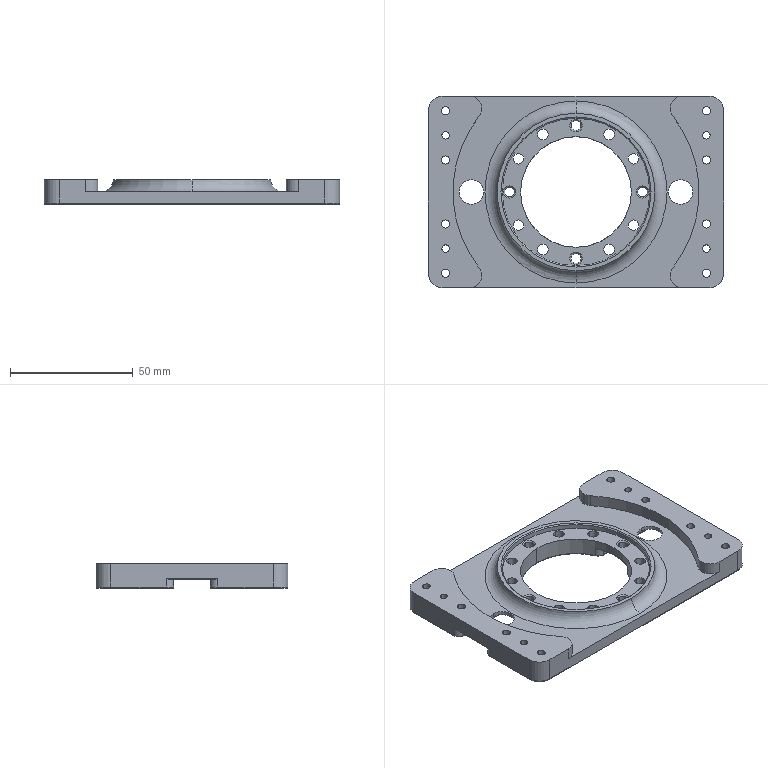NC program | NX | posted with a generic post | part box 120 x 78 x 10 mm
Whole program:
N10 G17 G21 G94 G90
(HOLE_MILLING_1_COPY_1 , TOOL : D3)
N12 T17 M6
N14 G54
N16 G17 G0 G90 X-47.5 Y0. B0. C0. S9500 M3
N18 G43 Z30. H17
N20 Z0.5
N22 G94 G3 X-47.95 Y0.45 R0.45 F1250.
N24 X-48.4 Y0. R0.45
N26 X-48.4 Y0. Z0.25 I0.9 J0.
N28 X-48.4 Y0. Z0. I0.9 J0.
N30 X-48.4 Y0. Z-0.25 I0.9 J0.
N32 X-48.4 Y0. Z-0.5 I0.9 J0.
N34 X-48.4 Y0. Z-0.75 I0.9 J0.
N36 X-48.4 Y0. Z-1. I0.9 J0.
N38 X-48.4 Y0. Z-1.25 I0.9 J0.
N40 X-48.4 Y0. Z-1.5 I0.9 J0.
N42 X-48.4 Y0. Z-1.75 I0.9 J0.
N44 X-48.4 Y0. Z-2. I0.9 J0.
N46 X-48.4 Y0. Z-2.25 I0.9 J0.
N48 X-48.4 Y0. Z-2.5 I0.9 J0.
N50 X-48.4 Y0. Z-2.75 I0.9 J0.
N52 X-48.4 Y0. Z-3. I0.9 J0.
N54 X-48.4 Y0. Z-3.25 I0.9 J0.
N56 X-48.4 Y0. Z-3.5 I0.9 J0.
N58 X-48.4 Y0. Z-3.75 I0.9 J0.
N60 X-48.4 Y0. Z-4. I0.9 J0.
N62 X-48.4 Y0. Z-4.25 I0.9 J0.
N64 X-48.4 Y0. Z-4.5 I0.9 J0.
N66 X-48.4 Y0. Z-4.75 I0.9 J0.
N68 X-48.4 Y0. Z-5. I0.9 J0.
N70 X-48.4 Y0. Z-5.25 I0.9 J0.
N72 X-48.4 Y0. Z-5.5 I0.9 J0.
N74 X-48.4 Y0. Z-5.75 I0.9 J0.
N76 X-48.4 Y0. Z-6. I0.9 J0.
N78 X-48.4 Y0. Z-6.25 I0.9 J0.
N80 X-48.4 Y0. Z-6.5 I0.9 J0.
N82 X-48.4 Y0. Z-6.75 I0.9 J0.
N84 X-48.4 Y0. Z-7. I0.9 J0.
N86 X-48.4 Y0. Z-7.25 I0.9 J0.
N88 X-48.4 Y0. Z-7.5 I0.9 J0.
N90 X-48.4 Y0. Z-7.75 I0.9 J0.
N92 X-48.4 Y0. Z-8. I0.9 J0.
N94 X-48.4 Y0. Z-8.25 I0.9 J0.
N96 X-48.4 Y0. Z-8.5 I0.9 J0.
N98 X-48.4 Y0. Z-8.75 I0.9 J0.
N100 X-48.4 Y0. Z-9. I0.9 J0.
N102 X-48.4 Y0. Z-9.25 I0.9 J0.
N104 X-48.4 Y0. Z-9.5 I0.9 J0.
N106 X-48.4 Y0. Z-9.75 I0.9 J0.
N108 X-48.4 Y0. Z-10. I0.9 J0.
N110 X-47.5 Y-0.9 R0.9
N112 X-48.4 Y0. R-0.9
N114 X-47.95 Y-0.45 R0.45
N116 X-47.5 Y0. R0.45
N118 G0 Z30.
N120 X47.5
N122 Z0.5
N124 G3 X47.05 Y0.45 R0.45
N126 X46.6 Y0. R0.45
N128 X46.6 Y0. Z0.25 I0.9 J0.
N130 X46.6 Y0. Z0. I0.9 J0.
N132 X46.6 Y0. Z-0.25 I0.9 J0.
N134 X46.6 Y0. Z-0.5 I0.9 J0.
N136 X46.6 Y0. Z-0.75 I0.9 J0.
N138 X46.6 Y0. Z-1. I0.9 J0.
N140 X46.6 Y0. Z-1.25 I0.9 J0.
N142 X46.6 Y0. Z-1.5 I0.9 J0.
N144 X46.6 Y0. Z-1.75 I0.9 J0.
N146 X46.6 Y0. Z-2. I0.9 J0.
N148 X46.6 Y0. Z-2.25 I0.9 J0.
N150 X46.6 Y0. Z-2.5 I0.9 J0.
N152 X46.6 Y0. Z-2.75 I0.9 J0.
N154 X46.6 Y0. Z-3. I0.9 J0.
N156 X46.6 Y0. Z-3.25 I0.9 J0.
N158 X46.6 Y0. Z-3.5 I0.9 J0.
N160 X46.6 Y0. Z-3.75 I0.9 J0.
N162 X46.6 Y0. Z-4. I0.9 J0.
N164 X46.6 Y0. Z-4.25 I0.9 J0.
N166 X46.6 Y0. Z-4.5 I0.9 J0.
N168 X46.6 Y0. Z-4.75 I0.9 J0.
N170 X46.6 Y0. Z-5. I0.9 J0.
N172 X46.6 Y0. Z-5.25 I0.9 J0.
N174 X46.6 Y0. Z-5.5 I0.9 J0.
N176 X46.6 Y0. Z-5.75 I0.9 J0.
N178 X46.6 Y0. Z-6. I0.9 J0.
N180 X46.6 Y0. Z-6.25 I0.9 J0.
N182 X46.6 Y0. Z-6.5 I0.9 J0.
N184 X46.6 Y0. Z-6.75 I0.9 J0.
N186 X46.6 Y0. Z-7. I0.9 J0.
N188 X46.6 Y0. Z-7.25 I0.9 J0.
N190 X46.6 Y0. Z-7.5 I0.9 J0.
N192 X46.6 Y0. Z-7.75 I0.9 J0.
N194 X46.6 Y0. Z-8. I0.9 J0.
N196 X46.6 Y0. Z-8.25 I0.9 J0.
N198 X46.6 Y0. Z-8.5 I0.9 J0.
N200 X46.6 Y0. Z-8.75 I0.9 J0.
N202 X46.6 Y0. Z-9. I0.9 J0.
N204 X46.6 Y0. Z-9.25 I0.9 J0.
N206 X46.6 Y0. Z-9.5 I0.9 J0.
N208 X46.6 Y0. Z-9.75 I0.9 J0.
N210 X46.6 Y0. Z-10. I0.9 J0.
N212 X47.5 Y-0.9 R0.9
N214 X46.6 Y0. R-0.9
N216 X47.05 Y-0.45 R0.45
N218 X47.5 Y0. R0.45
N220 G0 Z30.
N222 M5
(ZLEVEL_PROFILE_COPY_1_COPY_COPY_1_COPY , TOOL : D6A45)
N224 T01 M6
N226 G54
N228 G17 G0 G90 X-46.138 Y1.38 B0. C0. S9500 M3
N230 G43 Z30. H1
N232 Z2.646
N234 G94 G1 Z-0.354 F1000.
N236 X-46.98 Y2.839
N238 G3 X-47.5 Y3.139 R0.6
N240 X-50.639 Y0. R3.139 F1200.
N242 X-47.5 Y3.139 R-3.139
N244 G1 X-47.731 Y3.123 Z-0.357
N246 X-47.961 Y3.098 Z-0.361
N248 X-48.187 Y3.048 Z-0.364
N250 X-48.41 Y2.989 Z-0.368
N252 X-48.626 Y2.907 Z-0.371
N254 X-48.837 Y2.817 Z-0.375
N256 X-49.038 Y2.704 Z-0.378
N258 X-49.234 Y2.583 Z-0.382
N260 X-49.415 Y2.443 Z-0.385
N262 X-49.59 Y2.294 Z-0.389
N264 X-49.749 Y2.129 Z-0.392
N266 X-49.9 Y1.957 Z-0.396
N268 X-50.032 Y1.771 Z-0.399
N270 X-50.156 Y1.579 Z-0.403
N272 X-50.259 Y1.375 Z-0.406
N274 X-50.353 Y1.168 Z-0.41
N276 X-50.424 Y0.952 Z-0.413
N278 X-50.487 Y0.733 Z-0.417
N280 X-50.536 Y0.47 Z-0.421
N282 X-50.556 Y0.285 Z-0.423
N284 X-50.561 Y0.059 Z-0.427
N286 X-50.558 Y-0.168 Z-0.43
N288 X-50.53 Y-0.392 Z-0.434
N290 X-50.493 Y-0.615 Z-0.437
N292 X-50.432 Y-0.832 Z-0.441
N294 X-50.363 Y-1.046 Z-0.444
N296 X-50.271 Y-1.254 Z-0.448
N298 X-50.169 Y-1.458 Z-0.451
N300 X-50.047 Y-1.65 Z-0.455
N302 X-49.917 Y-1.836 Z-0.458
N304 X-49.767 Y-2.006 Z-0.461
N306 X-49.611 Y-2.17 Z-0.465
N308 X-49.439 Y-2.316 Z-0.468
N310 X-49.26 Y-2.455 Z-0.472
N312 X-49.068 Y-2.573 Z-0.475
N314 X-48.872 Y-2.684 Z-0.479
N316 X-48.664 Y-2.772 Z-0.482
N318 X-48.454 Y-2.852 Z-0.486
N320 X-48.237 Y-2.908 Z-0.489
N322 X-48.017 Y-2.955 Z-0.492
N324 X-47.794 Y-2.979 Z-0.496
N326 X-47.571 Y-2.993 Z-0.499
N328 X-47.348 Y-2.983 Z-0.503
N330 X-47.125 Y-2.963 Z-0.506
N332 X-46.906 Y-2.919 Z-0.509
N334 X-46.689 Y-2.868 Z-0.513
N336 X-46.424 Y-2.774 Z-0.517
N338 X-46.274 Y-2.708 Z-0.52
N340 X-46.079 Y-2.603 Z-0.523
N342 X-45.887 Y-2.49 Z-0.526
N344 X-45.711 Y-2.356 Z-0.53
N346 X-45.539 Y-2.217 Z-0.533
N348 X-45.384 Y-2.059 Z-0.537
N350 X-45.235 Y-1.895 Z-0.54
N352 X-45.106 Y-1.717 Z-0.543
N354 X-44.984 Y-1.533 Z-0.547
N356 X-44.883 Y-1.338 Z-0.55
N358 X-44.79 Y-1.138 Z-0.553
N360 X-44.719 Y-0.93 Z-0.557
N362 X-44.657 Y-0.72 Z-0.56
N364 X-44.619 Y-0.504 Z-0.563
N366 X-44.588 Y-0.288 Z-0.567
N368 X-44.582 Y-0.069 Z-0.57
N370 X-44.584 Y0.149 Z-0.573
N372 X-44.611 Y0.366 Z-0.577
N374 X-44.646 Y0.581 Z-0.58
N376 X-44.704 Y0.79 Z-0.583
N378 X-44.77 Y0.998 Z-0.587
N380 X-44.859 Y1.196 Z-0.59
N382 X-44.955 Y1.39 Z-0.593
N384 X-45.072 Y1.572 Z-0.597
N386 X-45.196 Y1.75 Z-0.6
N388 X-45.339 Y1.912 Z-0.603
N390 X-45.487 Y2.069 Z-0.606
N392 X-45.694 Y2.246 Z-0.611
N394 X-45.822 Y2.34 Z-0.613
N396 X-46.005 Y2.453 Z-0.616
N398 X-46.192 Y2.559 Z-0.62
N400 X-46.39 Y2.642 Z-0.623
N402 X-46.59 Y2.719 Z-0.626
N404 X-46.798 Y2.772 Z-0.629
N406 X-47.007 Y2.817 Z-0.633
N408 X-47.253 Y2.846 Z-0.636
N410 X-47.5 Y2.853 Z-0.64
N412 X-47.723 Y2.836 Z-0.644
N414 X-47.946 Y2.81 Z-0.648
N416 X-48.164 Y2.759 Z-0.651
N418 X-48.379 Y2.698 Z-0.655
N420 X-48.585 Y2.613 Z-0.659
N422 X-48.788 Y2.52 Z-0.663
N424 X-48.978 Y2.404 Z-0.667
N426 X-49.163 Y2.281 Z-0.67
N428 X-49.332 Y2.137 Z-0.674
N430 X-49.494 Y1.987 Z-0.678
N432 X-49.638 Y1.819 Z-0.681
N434 X-49.775 Y1.645 Z-0.685
N436 X-49.891 Y1.457 Z-0.689
N438 X-49.998 Y1.264 Z-0.693
N440 X-50.083 Y1.061 Z-0.696
N442 X-50.159 Y0.855 Z-0.7
N444 X-50.21 Y0.641 Z-0.704
N446 X-50.253 Y0.426 Z-0.707
N448 X-50.267 Y0.305 Z-0.71
N450 X-50.273 Y0.142 Z-0.712
N452 X-50.278 Y-0.021 Z-0.715
N454 X-50.259 Y-0.243 Z-0.719
N456 X-50.231 Y-0.465 Z-0.723
N458 X-50.177 Y-0.681 Z-0.726
N460 X-50.114 Y-0.895 Z-0.73
N462 X-50.026 Y-1.099 Z-0.734
N464 X-49.93 Y-1.299 Z-0.738
N466 X-49.812 Y-1.486 Z-0.741
N468 X-49.684 Y-1.667 Z-0.745
N470 X-49.537 Y-1.832 Z-0.749
N472 X-49.383 Y-1.991 Z-0.752
N474 X-49.212 Y-2.129 Z-0.756
N476 X-49.035 Y-2.261 Z-0.76
N478 X-48.845 Y-2.37 Z-0.764
N480 X-48.65 Y-2.471 Z-0.767
N482 X-48.445 Y-2.548 Z-0.771
N484 X-48.236 Y-2.616 Z-0.775
N486 X-48.022 Y-2.66 Z-0.778
N488 X-47.806 Y-2.693 Z-0.782
N490 X-47.589 Y-2.701 Z-0.786
N492 X-47.371 Y-2.7 Z-0.789
N494 X-47.155 Y-2.673 Z-0.793
N496 X-46.941 Y-2.637 Z-0.797
N498 X-46.733 Y-2.577 Z-0.8
N500 X-46.528 Y-2.507 Z-0.804
N502 X-46.42 Y-2.46 Z-0.806
N504 X-46.28 Y-2.387 Z-0.809
N506 X-46.142 Y-2.312 Z-0.811
N508 X-45.965 Y-2.189 Z-0.815
N510 X-45.793 Y-2.059 Z-0.819
N512 X-45.639 Y-1.909 Z-0.822
N514 X-45.49 Y-1.753 Z-0.826
N516 X-45.362 Y-1.581 Z-0.83
N518 X-45.241 Y-1.404 Z-0.833
N520 X-45.142 Y-1.215 Z-0.837
N522 X-45.052 Y-1.021 Z-0.84
N524 X-44.985 Y-0.819 Z-0.844
N526 X-44.927 Y-0.614 Z-0.848
N528 X-44.893 Y-0.404 Z-0.851
N530 X-44.869 Y-0.192 Z-0.855
N532 Y0.02 Z-0.858
N534 X-44.879 Y0.232 Z-0.862
N536 X-44.914 Y0.44 Z-0.865
N538 X-44.957 Y0.647 Z-0.869
N540 X-45.024 Y0.847 Z-0.873
N542 X-45.1 Y1.044 Z-0.876
N544 X-45.199 Y1.23 Z-0.88
N546 X-45.305 Y1.411 Z-0.883
N548 X-45.432 Y1.579 Z-0.887
N550 X-45.565 Y1.741 Z-0.89
N552 X-45.716 Y1.885 Z-0.894
N554 X-45.874 Y2.023 Z-0.897
N556 X-45.965 Y2.09 Z-0.899
N558 X-46.165 Y2.219 Z-0.903
N560 X-46.321 Y2.298 Z-0.906
N562 X-46.479 Y2.373 Z-0.909
N564 X-46.644 Y2.43 Z-0.912
N566 X-46.81 Y2.484 Z-0.915
N568 X-46.981 Y2.518 Z-0.918
N570 X-47.153 Y2.548 Z-0.921
N572 X-47.326 Y2.559 Z-0.924
N574 X-47.5 Y2.566 Z-0.927
N576 X-47.659 Y2.554 Z-0.93
N578 X-47.818 Y2.54 Z-0.933
N580 X-47.913 Y2.525 Z-0.935
N582 X-48.115 Y2.475 Z-0.939
N584 X-48.314 Y2.417 Z-0.942
N586 X-48.503 Y2.336 Z-0.946
N588 X-48.69 Y2.247 Z-0.95
N590 X-48.864 Y2.137 Z-0.954
N592 X-49.033 Y2.019 Z-0.958
N594 X-49.186 Y1.882 Z-0.962
N596 X-49.333 Y1.739 Z-0.966
N598 X-49.462 Y1.58 Z-0.97
N600 X-49.584 Y1.416 Z-0.973
N602 X-49.685 Y1.239 Z-0.977
N604 X-49.778 Y1.057 Z-0.981
N606 X-49.849 Y0.867 Z-0.985
N608 X-49.912 Y0.673 Z-0.989
N610 X-49.951 Y0.474 Z-0.993
N612 X-49.981 Y0.274 Z-0.996
N614 X-49.992 Y0.116 Z-0.999
N616 X-49.991 Y-0.029 Z-1.002
N618 X-49.983 Y-0.161 Z-1.005
N620 X-49.952 Y-0.375 Z-1.009
N622 X-49.909 Y-0.588 Z-1.013
N624 X-49.866 Y-0.737 Z-1.016
N626 X-49.841 Y-0.811 Z-1.017
N628 X-49.816 Y-0.872 Z-1.018
N630 X-49.763 Y-0.994 Z-1.021
N632 X-49.661 Y-1.183 Z-1.025
N634 X-49.549 Y-1.367 Z-1.029
N636 X-49.462 Y-1.486 Z-1.032
N638 X-49.368 Y-1.591 Z-1.035
N640 X-49.275 Y-1.696 Z-1.037
N642 X-49.161 Y-1.805 Z-1.04
N644 X-49.102 Y-1.857 Z-1.042
N646 X-49.052 Y-1.897 Z-1.043
N648 X-48.949 Y-1.972 Z-1.045
N650 X-48.767 Y-2.084 Z-1.049
N652 X-48.58 Y-2.187 Z-1.053
N654 X-48.441 Y-2.248 Z-1.056
N656 X-48.308 Y-2.297 Z-1.059
N658 X-48.182 Y-2.333 Z-1.061
N660 X-47.975 Y-2.376 Z-1.065
N662 X-47.766 Y-2.408 Z-1.069
N664 X-47.614 Y-2.419 Z-1.072
N666 X-47.473 Z-1.075
N668 X-47.344 Y-2.41 Z-1.077
N670 X-47.136 Y-2.38 Z-1.081
N672 X-46.93 Y-2.339 Z-1.085
N674 X-46.784 Y-2.296 Z-1.088
N676 X-46.713 Y-2.272 Z-1.09
N678 X-46.653 Y-2.248 Z-1.091
N680 X-46.535 Y-2.197 Z-1.093
N682 X-46.352 Y-2.098 Z-1.097
N684 X-46.173 Y-1.989 Z-1.101
N686 X-46.052 Y-1.901 Z-1.104
N688 X-45.946 Y-1.812 Z-1.106
N690 X-45.853 Y-1.723 Z-1.109
N692 X-45.715 Y-1.568 Z-1.113
N694 X-45.585 Y-1.406 Z-1.117
N696 X-45.477 Y-1.23 Z-1.121
N698 X-45.377 Y-1.049 Z-1.125
N700 X-45.321 Y-0.919 Z-1.127
N702 X-45.277 Y-0.791 Z-1.13
N704 X-45.235 Y-0.662 Z-1.132
N706 X-45.198 Y-0.515 Z-1.135
N708 X-45.184 Y-0.44 Z-1.137
N710 X-45.175 Y-0.38 Z-1.138
N712 X-45.162 Y-0.258 Z-1.14
N714 X-45.156 Y-0.053 Z-1.144
N716 X-45.161 Y0.152 Z-1.148
N718 X-45.176 Y0.298 Z-1.151
N720 X-45.199 Y0.432 Z-1.153
N722 X-45.23 Y0.554 Z-1.155
N724 X-45.293 Y0.747 Z-1.159
N726 X-45.368 Y0.936 Z-1.163
N728 X-45.432 Y1.069 Z-1.166
N730 X-45.5 Y1.186 Z-1.168
N732 X-45.569 Y1.288 Z-1.171
N734 X-45.694 Y1.447 Z-1.175
N736 X-45.828 Y1.599 Z-1.178
N738 X-45.978 Y1.733 Z-1.182
N740 X-46.135 Y1.859 Z-1.186
N742 X-46.29 Y1.955 Z-1.189
N744 X-46.448 Y2.044 Z-1.193
N746 X-46.616 Y2.115 Z-1.196
N748 X-46.786 Y2.178 Z-1.2
N750 X-46.962 Y2.222 Z-1.203
N752 X-47.14 Y2.257 Z-1.207
N754 X-47.32 Y2.271 Z-1.21
N756 X-47.5 Y2.279 Z-1.213
N758 X-47.641 Y2.268 Z-1.216
N760 X-47.782 Y2.255 Z-1.219
N762 X-47.926 Y2.231 Z-1.223
N764 X-48.054 Y2.2 Z-1.225
N766 X-48.167 Y2.164 Z-1.228
N768 X-48.35 Y2.09 Z-1.232
N770 X-48.529 Y2.007 Z-1.236
N772 X-48.587 Y1.975 Z-1.238
N774 X-48.723 Y1.886 Z-1.241
N776 X-48.857 Y1.792 Z-1.245
N778 X-48.968 Y1.7 Z-1.248
N780 X-49.062 Y1.61 Z-1.251
N782 X-49.141 Y1.523 Z-1.253
N784 X-49.262 Y1.37 Z-1.257
N786 X-49.374 Y1.21 Z-1.261
N788 X-49.445 Y1.089 Z-1.264
N790 X-49.477 Y1.027 Z-1.266
N792 X-49.502 Y0.973 Z-1.267
N794 X-49.548 Y0.863 Z-1.27
N796 X-49.608 Y0.68 Z-1.274
N798 X-49.659 Y0.493 Z-1.278
N800 X-49.684 Y0.357 Z-1.281
N802 X-49.698 Y0.229 Z-1.284
N804 X-49.703 Y0.11 Z-1.286
N806 X-49.697 Y-0.082 Z-1.29
N808 X-49.681 Y-0.273 Z-1.295
N810 X-49.658 Y-0.409 Z-1.297
N812 X-49.628 Y-0.533 Z-1.3
N814 X-49.592 Y-0.645 Z-1.303
N816 X-49.521 Y-0.822 Z-1.307
N818 X-49.441 Y-0.995 Z-1.311
N820 X-49.374 Y-1.114 Z-1.314
N822 X-49.337 Y-1.172 Z-1.315
N824 X-49.303 Y-1.219 Z-1.316
N826 X-49.233 Y-1.312 Z-1.319
N828 X-49.106 Y-1.453 Z-1.323
N830 X-48.973 Y-1.587 Z-1.327
N832 X-48.825 Y-1.703 Z-1.331
N834 X-48.671 Y-1.812 Z-1.335
N836 X-48.616 Y-1.845 Z-1.337
N838 X-48.476 Y-1.914 Z-1.34
N840 X-48.335 Y-1.98 Z-1.343
N842 X-48.208 Y-2.028 Z-1.346
N844 X-48.088 Y-2.063 Z-1.349
N846 X-47.977 Y-2.088 Z-1.351
N848 X-47.792 Y-2.113 Z-1.355
N850 X-47.606 Y-2.131 Z-1.359
N852 X-47.474 Z-1.362
N854 X-47.407 Y-2.128 Z-1.363
N856 X-47.35 Y-2.123 Z-1.365
N858 X-47.236 Y-2.109 Z-1.367
N860 X-47.055 Y-2.07 Z-1.371
N862 X-46.876 Y-2.023 Z-1.375
N864 X-46.692 Y-1.954 Z-1.379
N866 X-46.538 Y-1.877 Z-1.383
N868 X-46.382 Y-1.78 Z-1.387
N870 X-46.231 Y-1.675 Z-1.391
N872 X-46.083 Y-1.548 Z-1.395
N874 X-45.965 Y-1.424 Z-1.399
N876 X-45.853 Y-1.281 Z-1.403
N878 X-45.748 Y-1.132 Z-1.406
N880 X-45.682 Y-1.019 Z-1.409
N882 X-45.652 Y-0.962 Z-1.411
N884 X-45.628 Y-0.911 Z-1.412
N886 X-45.585 Y-0.807 Z-1.414
N888 X-45.528 Y-0.631 Z-1.418
N890 X-45.479 Y-0.452 Z-1.422
N892 X-45.455 Y-0.268 Z-1.426
N894 X-45.439 Y-0.084 Z-1.43
N896 Y-0.042 Z-1.431
N898 X-45.449 Y0.121 Z-1.435
N900 X-45.465 Y0.283 Z-1.438
N902 X-45.489 Y0.412 Z-1.441
N904 X-45.504 Y0.476 Z-1.442
N906 X-45.52 Y0.531 Z-1.443
N908 X-45.555 Y0.639 Z-1.446
N910 X-45.628 Y0.806 Z-1.45
N912 X-45.707 Y0.971 Z-1.454
N914 X-45.81 Y1.135 Z-1.458
N916 X-45.915 Y1.27 Z-1.462
N918 X-46.04 Y1.401 Z-1.465
N920 X-46.171 Y1.526 Z-1.469
N922 X-46.325 Y1.644 Z-1.473
N924 X-46.468 Y1.732 Z-1.477
N926 X-46.631 Y1.81 Z-1.481
N928 X-46.796 Y1.881 Z-1.485
N930 X-46.978 Y1.935 Z-1.489
N932 X-47.144 Y1.969 Z-1.492
N934 X-47.321 Y1.985 Z-1.496
N936 X-47.5 Y1.993 Z-1.5
N938 G3 X-49.493 Y0. R1.993
N940 X-47.5 Y1.993 R-1.993
N942 X-48.02 Y1.693 R0.6
N944 G1 X-47.733 Y0.758
N946 Z1.5
N948 G0 Z30.
N950 X46.138 Y-1.381
N952 Z2.646
N954 G1 Z-0.354 F1000.
N956 X46.98 Y-2.839
N958 G3 X47.5 Y-3.139 R0.6
N960 X50.639 Y0. R3.139 F1200.
N962 X47.5 Y-3.139 R-3.139
N964 G1 X47.728 Y-3.123 Z-0.357
N966 X47.955 Y-3.099 Z-0.361
N968 X48.177 Y-3.05 Z-0.364
N970 X48.398 Y-2.994 Z-0.367
N972 X48.629 Y-2.91 Z-0.371
N974 X48.82 Y-2.825 Z-0.374
N976 X49.018 Y-2.715 Z-0.378
N978 X49.212 Y-2.598 Z-0.381
N980 X49.392 Y-2.461 Z-0.385
N982 X49.566 Y-2.317 Z-0.388
N984 X49.724 Y-2.156 Z-0.392
N986 X49.876 Y-1.988 Z-0.395
N988 X50.012 Y-1.801 Z-0.399
N990 X50.139 Y-1.608 Z-0.402
N992 X50.246 Y-1.403 Z-0.406
N994 X50.343 Y-1.194 Z-0.409
N996 X50.417 Y-0.976 Z-0.413
N998 X50.482 Y-0.755 Z-0.416
N1000 X50.523 Y-0.529 Z-0.42
N1002 X50.555 Y-0.302 Z-0.423
N1004 X50.561 Y-0.073 Z-0.427
N1006 X50.559 Y0.157 Z-0.43
N1008 X50.531 Y0.384 Z-0.434
N1010 X50.494 Y0.609 Z-0.437
N1012 X50.433 Y0.829 Z-0.441
N1014 X50.363 Y1.046 Z-0.444
N1016 X50.271 Y1.254 Z-0.448
N1018 X50.169 Y1.458 Z-0.451
N1020 X50.047 Y1.65 Z-0.455
N1022 X49.917 Y1.836 Z-0.458
N1024 X49.767 Y2.006 Z-0.461
N1026 X49.611 Y2.17 Z-0.465
N1028 X49.394 Y2.356 Z-0.469
N1030 X49.26 Y2.455 Z-0.472
N1032 X49.068 Y2.573 Z-0.475
N1034 X48.872 Y2.684 Z-0.479
N1036 X48.664 Y2.772 Z-0.482
N1038 X48.454 Y2.852 Z-0.486
N1040 X48.237 Y2.908 Z-0.489
N1042 X48.017 Y2.955 Z-0.492
N1044 X47.794 Y2.979 Z-0.496
N1046 X47.571 Y2.993 Z-0.499
N1048 X47.348 Y2.983 Z-0.503
N1050 X47.125 Y2.963 Z-0.506
N1052 X46.906 Y2.919 Z-0.509
N1054 X46.689 Y2.868 Z-0.513
N1056 X46.48 Y2.792 Z-0.516
N1058 X46.274 Y2.708 Z-0.52
N1060 X46.079 Y2.603 Z-0.523
N1062 X45.887 Y2.49 Z-0.526
N1064 X45.711 Y2.356 Z-0.53
N1066 X45.539 Y2.217 Z-0.533
N1068 X45.384 Y2.059 Z-0.537
N1070 X45.235 Y1.895 Z-0.54
N1072 X45.106 Y1.717 Z-0.543
N1074 X44.984 Y1.533 Z-0.547
N1076 X44.883 Y1.338 Z-0.55
N1078 X44.79 Y1.138 Z-0.553
N1080 X44.719 Y0.93 Z-0.557
N1082 X44.657 Y0.72 Z-0.56
N1084 X44.606 Y0.448 Z-0.564
N1086 X44.588 Y0.288 Z-0.567
N1088 X44.582 Y0.069 Z-0.57
N1090 X44.584 Y-0.149 Z-0.573
N1092 X44.611 Y-0.366 Z-0.577
N1094 X44.646 Y-0.581 Z-0.58
N1096 X44.704 Y-0.79 Z-0.583
N1098 X44.77 Y-0.998 Z-0.587
N1100 X44.861 Y-1.2 Z-0.59
N1102 X44.96 Y-1.397 Z-0.593
N1104 X45.079 Y-1.583 Z-0.597
N1106 X45.207 Y-1.763 Z-0.6
N1108 X45.353 Y-1.928 Z-0.603
N1110 X45.506 Y-2.086 Z-0.607
N1112 X45.675 Y-2.226 Z-0.61
N1114 X45.85 Y-2.36 Z-0.614
N1116 X46.038 Y-2.472 Z-0.617
N1118 X46.231 Y-2.577 Z-0.62
N1120 X46.433 Y-2.66 Z-0.624
N1122 X46.639 Y-2.734 Z-0.627
N1124 X46.851 Y-2.784 Z-0.63
N1126 X47.066 Y-2.826 Z-0.634
N1128 X47.282 Y-2.843 Z-0.637
N1130 X47.5 Y-2.853 Z-0.64
N1132 X47.675 Y-2.84 Z-0.643
N1134 X47.85 Y-2.825 Z-0.646
N1136 X48.022 Y-2.791 Z-0.649
N1138 X48.194 Y-2.755 Z-0.652
N1140 X48.36 Y-2.7 Z-0.655
N1142 X48.525 Y-2.643 Z-0.658
N1144 X48.639 Y-2.594 Z-0.66
N1146 X48.786 Y-2.517 Z-0.663
N1148 X48.932 Y-2.438 Z-0.666
N1150 X49.119 Y-2.308 Z-0.669
N1152 X49.3 Y-2.171 Z-0.673
N1154 X49.463 Y-2.013 Z-0.677
N1156 X49.619 Y-1.849 Z-0.681
N1158 X49.754 Y-1.668 Z-0.685
N1160 X49.881 Y-1.481 Z-0.689
N1162 X49.986 Y-1.281 Z-0.692
N1164 X50.081 Y-1.077 Z-0.696
N1166 X50.152 Y-0.863 Z-0.7
N1168 X50.213 Y-0.647 Z-0.704
N1170 X50.249 Y-0.426 Z-0.707
N1172 X50.274 Y-0.203 Z-0.711
N1174 Y0.021 Z-0.715
N1176 X50.263 Y0.244 Z-0.719
N1178 X50.227 Y0.464 Z-0.723
N1180 X50.181 Y0.682 Z-0.726
N1182 X50.11 Y0.893 Z-0.73
N1184 X50.03 Y1.101 Z-0.734
N1186 X49.926 Y1.297 Z-0.738
N1188 X49.814 Y1.488 Z-0.741
N1190 X49.681 Y1.665 Z-0.745
N1192 X49.54 Y1.835 Z-0.749
N1194 X49.381 Y1.988 Z-0.752
N1196 X49.215 Y2.133 Z-0.756
N1198 X49.119 Y2.204 Z-0.758
N1200 X48.983 Y2.29 Z-0.761
N1202 X48.847 Y2.374 Z-0.764
N1204 X48.648 Y2.467 Z-0.767
N1206 X48.446 Y2.552 Z-0.771
N1208 X48.236 Y2.612 Z-0.775
N1210 X48.023 Y2.664 Z-0.778
N1212 X47.806 Y2.689 Z-0.782
N1214 X47.589 Y2.706 Z-0.786
N1216 X47.371 Y2.697 Z-0.789
N1218 X47.154 Y2.678 Z-0.793
N1220 X46.942 Y2.633 Z-0.797
N1222 X46.731 Y2.58 Z-0.8
N1224 X46.529 Y2.503 Z-0.804
N1226 X46.331 Y2.417 Z-0.808
N1228 X46.144 Y2.309 Z-0.811
N1230 X45.962 Y2.192 Z-0.815
N1232 X45.796 Y2.055 Z-0.819
N1234 X45.636 Y1.912 Z-0.822
N1236 X45.494 Y1.751 Z-0.826
N1238 X45.359 Y1.584 Z-0.83
N1240 X45.245 Y1.403 Z-0.833
N1242 X45.139 Y1.217 Z-0.837
N1244 X45.056 Y1.02 Z-0.84
N1246 X44.981 Y0.82 Z-0.844
N1248 X44.931 Y0.613 Z-0.848
N1250 X44.889 Y0.404 Z-0.851
N1252 X44.876 Y0.289 Z-0.853
N1254 X44.87 Y0.141 Z-0.856
N1256 X44.865 Y-0.008 Z-0.858
N1258 X44.882 Y-0.214 Z-0.862
N1260 X44.906 Y-0.419 Z-0.865
N1262 X44.953 Y-0.618 Z-0.869
N1264 X45.009 Y-0.816 Z-0.872
N1266 X45.088 Y-1.006 Z-0.875
N1268 X45.174 Y-1.192 Z-0.879
N1270 X45.281 Y-1.366 Z-0.882
N1272 X45.394 Y-1.536 Z-0.886
N1274 X45.526 Y-1.692 Z-0.889
N1276 X45.664 Y-1.842 Z-0.893
N1278 X45.819 Y-1.974 Z-0.896
N1280 X45.978 Y-2.1 Z-0.9
N1282 X46.151 Y-2.206 Z-0.903
N1284 X46.328 Y-2.306 Z-0.906
N1286 X46.515 Y-2.383 Z-0.91
N1288 X46.704 Y-2.454 Z-0.913
N1290 X46.9 Y-2.502 Z-0.917
N1292 X47.098 Y-2.541 Z-0.92
N1294 X47.299 Y-2.557 Z-0.923
N1296 X47.5 Y-2.566 Z-0.927
N1298 X47.676 Y-2.552 Z-0.93
N1300 X47.852 Y-2.535 Z-0.933
N1302 X48.024 Y-2.497 Z-0.937
N1304 X48.195 Y-2.456 Z-0.94
N1306 X48.36 Y-2.395 Z-0.943
N1308 X48.524 Y-2.331 Z-0.947
N1310 X48.668 Y-2.26 Z-0.95
N1312 X48.796 Y-2.186 Z-0.953
N1314 X48.908 Y-2.111 Z-0.955
N1316 X49.082 Y-1.974 Z-0.959
N1318 X49.248 Y-1.828 Z-0.963
N1320 X49.357 Y-1.714 Z-0.966
N1322 X49.409 Y-1.654 Z-0.968
N1324 X49.452 Y-1.601 Z-0.969
N1326 X49.532 Y-1.492 Z-0.972
N1328 X49.647 Y-1.305 Z-0.976
N1330 X49.753 Y-1.113 Z-0.98
N1332 X49.813 Y-0.975 Z-0.983
N1334 X49.859 Y-0.839 Z-0.986
N1336 X49.904 Y-0.703 Z-0.988
N1338 X49.942 Y-0.547 Z-0.991
N1340 X49.957 Y-0.468 Z-0.993
N1342 X49.967 Y-0.404 Z-0.994
N1344 X49.981 Y-0.274 Z-0.996
N1346 X49.987 Y-0.056 Z-1.001
N1348 X49.983 Y0.161 Z-1.005
N1350 X49.966 Y0.316 Z-1.008
N1352 X49.941 Y0.458 Z-1.01
N1354 X49.909 Y0.588 Z-1.013
N1356 X49.841 Y0.793 Z-1.017
N1358 X49.763 Y0.994 Z-1.021
N1360 X49.695 Y1.133 Z-1.024
N1362 X49.623 Y1.257 Z-1.027
N1364 X49.549 Y1.367 Z-1.029
N1366 X49.416 Y1.535 Z-1.033
N1368 X49.275 Y1.697 Z-1.037
N1370 X49.164 Y1.803 Z-1.04
N1372 X49.106 Y1.854 Z-1.042
N1374 X49.054 Y1.895 Z-1.043
N1376 X48.949 Y1.972 Z-1.045
N1378 X48.767 Y2.084 Z-1.049
N1380 X48.58 Y2.187 Z-1.053
N1382 X48.441 Y2.248 Z-1.056
N1384 X48.308 Y2.297 Z-1.059
N1386 X48.182 Y2.333 Z-1.061
N1388 X47.975 Y2.376 Z-1.065
N1390 X47.766 Y2.409 Z-1.069
N1392 X47.555 Y2.415 Z-1.073
N1394 X47.344 Y2.41 Z-1.077
N1396 X47.2 Y2.394 Z-1.08
N1398 X47.065 Y2.366 Z-1.083
N1400 X46.93 Y2.339 Z-1.085
N1402 X46.782 Y2.296 Z-1.088
N1404 X46.709 Y2.271 Z-1.09
N1406 X46.651 Y2.248 Z-1.091
N1408 X46.535 Y2.197 Z-1.093
N1410 X46.352 Y2.098 Z-1.097
N1412 X46.173 Y1.989 Z-1.101
N1414 X46.052 Y1.901 Z-1.104
N1416 X45.946 Y1.812 Z-1.106
N1418 X45.853 Y1.723 Z-1.109
N1420 X45.715 Y1.568 Z-1.113
N1422 X45.585 Y1.406 Z-1.117
N1424 X45.501 Y1.282 Z-1.12
N1426 X45.433 Y1.163 Z-1.122
N1428 X45.377 Y1.049 Z-1.125
N1430 X45.301 Y0.857 Z-1.128
N1432 X45.235 Y0.662 Z-1.132
N1434 X45.199 Y0.519 Z-1.135
N1436 X45.185 Y0.447 Z-1.136
N1438 X45.176 Y0.384 Z-1.138
N1440 X45.162 Y0.258 Z-1.14
N1442 X45.156 Y0.061 Z-1.144
N1444 X45.159 Y-0.136 Z-1.147
N1446 X45.186 Y-0.331 Z-1.151
N1448 X45.222 Y-0.524 Z-1.155
N1450 X45.281 Y-0.711 Z-1.159
N1452 X45.349 Y-0.895 Z-1.162
N1454 X45.438 Y-1.069 Z-1.166
N1456 X45.535 Y-1.238 Z-1.17
N1458 X45.652 Y-1.4 Z-1.173
N1460 X45.776 Y-1.545 Z-1.177
N1462 X45.916 Y-1.679 Z-1.181
N1464 X46.063 Y-1.806 Z-1.184
N1466 X46.223 Y-1.914 Z-1.188
N1468 X46.389 Y-2.014 Z-1.192
N1470 X46.564 Y-2.094 Z-1.195
N1472 X46.744 Y-2.165 Z-1.199
N1474 X46.929 Y-2.214 Z-1.203
N1476 X47.118 Y-2.254 Z-1.206
N1478 X47.308 Y-2.271 Z-1.21
N1480 X47.5 Y-2.278 Z-1.213
N1482 X47.69 Y-2.263 Z-1.217
N1484 X47.878 Y-2.239 Z-1.222
N1486 X48.062 Y-2.192 Z-1.226
N1488 X48.243 Y-2.137 Z-1.23
N1490 X48.416 Y-2.06 Z-1.234
N1492 X48.585 Y-1.976 Z-1.238
N1494 X48.742 Y-1.872 Z-1.242
N1496 X48.894 Y-1.761 Z-1.246
N1498 X49.031 Y-1.633 Z-1.25
N1500 X49.162 Y-1.499 Z-1.254
N1502 X49.276 Y-1.35 Z-1.258
N1504 X49.382 Y-1.197 Z-1.262
N1506 X49.45 Y-1.08 Z-1.265
N1508 X49.481 Y-1.02 Z-1.266
N1510 X49.504 Y-0.969 Z-1.267
N1512 X49.548 Y-0.863 Z-1.27
N1514 X49.608 Y-0.68 Z-1.274
N1516 X49.659 Y-0.493 Z-1.278
N1518 X49.686 Y-0.302 Z-1.282
N1520 X49.703 Y-0.11 Z-1.286
N1522 X49.704 Y-0.045 Z-1.288
N1524 X49.695 Y0.114 Z-1.291
N1526 X49.681 Y0.273 Z-1.295
N1528 X49.658 Y0.411 Z-1.297
N1530 X49.627 Y0.535 Z-1.3
N1532 X49.592 Y0.645 Z-1.303
N1534 X49.521 Y0.822 Z-1.307
N1536 X49.441 Y0.995 Z-1.311
N1538 X49.374 Y1.114 Z-1.314
N1540 X49.337 Y1.172 Z-1.315
N1542 X49.303 Y1.219 Z-1.316
N1544 X49.233 Y1.312 Z-1.319
N1546 X49.106 Y1.453 Z-1.323
N1548 X48.973 Y1.587 Z-1.327
N1550 X48.87 Y1.674 Z-1.33
N1552 X48.769 Y1.749 Z-1.333
N1554 X48.671 Y1.812 Z-1.335
N1556 X48.505 Y1.9 Z-1.339
N1558 X48.335 Y1.98 Z-1.343
N1560 X48.21 Y2.027 Z-1.346
N1562 X48.09 Y2.062 Z-1.349
N1564 X47.977 Y2.088 Z-1.351
N1566 X47.792 Y2.113 Z-1.355
N1568 X47.606 Y2.131 Z-1.359
N1570 X47.474 Z-1.362
N1572 X47.407 Y2.128 Z-1.363
N1574 X47.35 Y2.123 Z-1.365
N1576 X47.236 Y2.109 Z-1.367
N1578 X47.055 Y2.07 Z-1.371
N1580 X46.876 Y2.023 Z-1.375
N1582 X46.705 Y1.954 Z-1.379
N1584 X46.538 Y1.877 Z-1.383
N1586 X46.483 Y1.847 Z-1.384
N1588 X46.356 Y1.763 Z-1.388
N1590 X46.231 Y1.675 Z-1.391
N1592 X46.081 Y1.546 Z-1.395
N1594 X45.965 Y1.424 Z-1.399
N1596 X45.853 Y1.281 Z-1.403
N1598 X45.748 Y1.132 Z-1.406
N1600 X45.652 Y0.963 Z-1.411
N1602 X45.585 Y0.807 Z-1.414
N1604 X45.53 Y0.635 Z-1.418
N1606 X45.481 Y0.461 Z-1.422
N1608 X45.45 Y0.272 Z-1.426
N1610 X45.44 Y0.103 Z-1.43
N1612 X45.446 Y-0.076 Z-1.434
N1614 X45.461 Y-0.255 Z-1.437
N1616 X45.496 Y-0.442 Z-1.441
N1618 X45.543 Y-0.603 Z-1.445
N1620 X45.61 Y-0.768 Z-1.449
N1622 X45.684 Y-0.931 Z-1.453
N1624 X45.782 Y-1.095 Z-1.457
N1626 X45.88 Y-1.227 Z-1.46
N1628 X46.006 Y-1.365 Z-1.464
N1630 X46.138 Y-1.498 Z-1.468
N1632 X46.293 Y-1.621 Z-1.473
N1634 X46.44 Y-1.716 Z-1.476
N1636 X46.631 Y-1.815 Z-1.481
N1638 X46.775 Y-1.874 Z-1.484
N1640 X46.953 Y-1.924 Z-1.488
N1642 X47.133 Y-1.967 Z-1.492
N1644 X47.316 Y-1.984 Z-1.496
N1646 X47.5 Y-1.993 Z-1.5
N1648 G3 X49.493 Y0. R1.993
N1650 X47.5 Y-1.993 R-1.993
N1652 X48.02 Y-1.693 R0.6
N1654 G1 X47.733 Y-0.758
N1656 Z1.5
N1658 G0 Z30.
N1660 M5
(刀补17_COPY , TOOL : D3)
N1662 T17 M6
N1664 G54
N1666 G17 G0 G90 X-47.5 Y0. B0. C0. S9500 M3
N1668 G43 Z30. H17
N1670 Z0.5
N1672 G41 G94 G1 X-47.504 Y0.1 F1250. D17
N1674 G3 X-48.45 Y0. R0.478
N1676 X-48.45 Y0. Z-2. I0.95 J0.
N1678 X-48.45 Y0. Z-4.5 I0.95 J0.
N1680 X-48.45 Y0. Z-7. I0.95 J0.
N1682 X-48.45 Y0. Z-9.5 I0.95 J0.
N1684 X-47.794 Y-0.904 Z-10. R0.95
N1686 X-46.596 Y-0.294 R0.95
N1688 X-47.794 Y-0.904 R-0.95
N1690 X-47.406 Y-0.034 R0.478
N1692 G40
N1694 G1 X-47.5 Y0.
N1696 G0 Z30.
N1698 X47.5
N1700 Z0.5
N1702 G41 G1 X47.496 Y0.1
N1704 G3 X46.55 Y0. R0.478
N1706 X46.55 Y0. Z-2. I0.95 J0.
N1708 X46.55 Y0. Z-4.5 I0.95 J0.
N1710 X46.55 Y0. Z-7. I0.95 J0.
N1712 X46.55 Y0. Z-9.5 I0.95 J0.
N1714 X47.206 Y-0.904 Z-10. R0.95
N1716 X48.404 Y-0.294 R0.95
N1718 X47.206 Y-0.904 R-0.95
N1720 X47.594 Y-0.034 R0.478
N1722 G40
N1724 G1 X47.5 Y0.
N1726 G0 Z30.
N1728 M5
N1730 M2